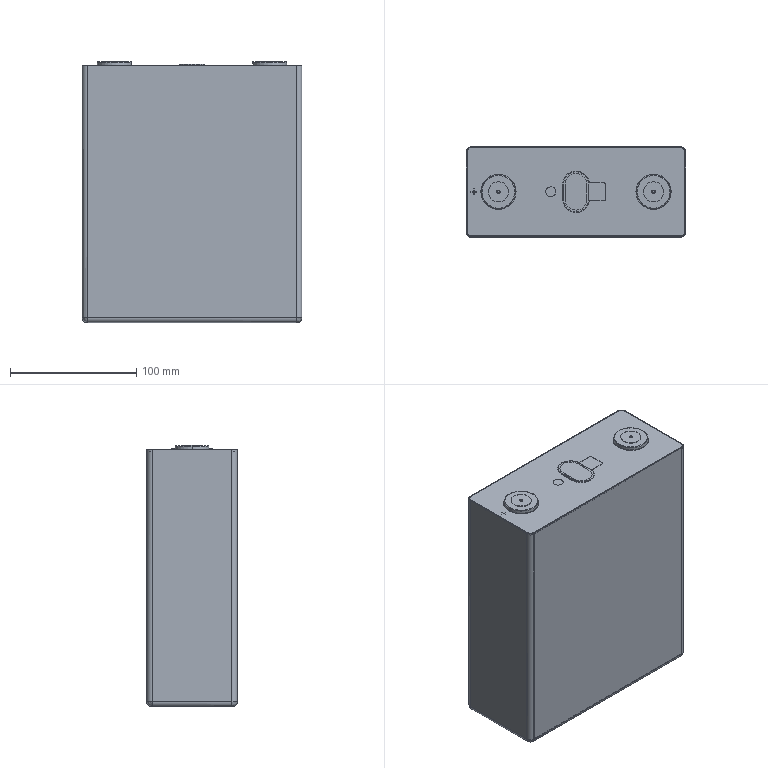Part | NX | features BREP 10 | 10 solids | 782 faces | box 173.9 x 71.65 x 207.3 mm | volume 147203 mm3 | cylinder 338 | plane 314 | torus 70 | cone 40 | spline 16 | sphere 4 | commonest cylinder face diameters 3 x72 1 x42 6 x34 2 x12 8 x12 16.6 x12